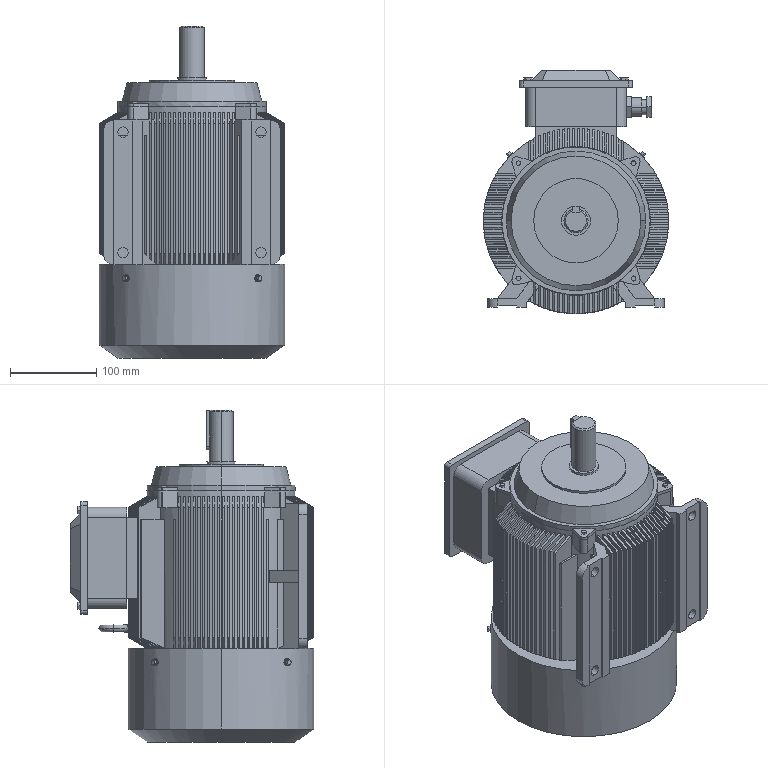Part | SolidWorks | features ICE 22, CirPattern 4, Revolution 4, Fillet 3, MoveCopyBody 3, Chamfer 2, PLine 2, DeleteBody 1, LPattern 1, SketchPattern 1 | 2 solids | 837 faces | box 215 x 282.5 x 385 mm | volume 11501075 mm3 | plane 403 | cone 275 | cylinder 155 | torus 4 | commonest cylinder face diameters 215 x84 10.75 x12 12 x12 8.6 x10 172 x9 7.83 x4